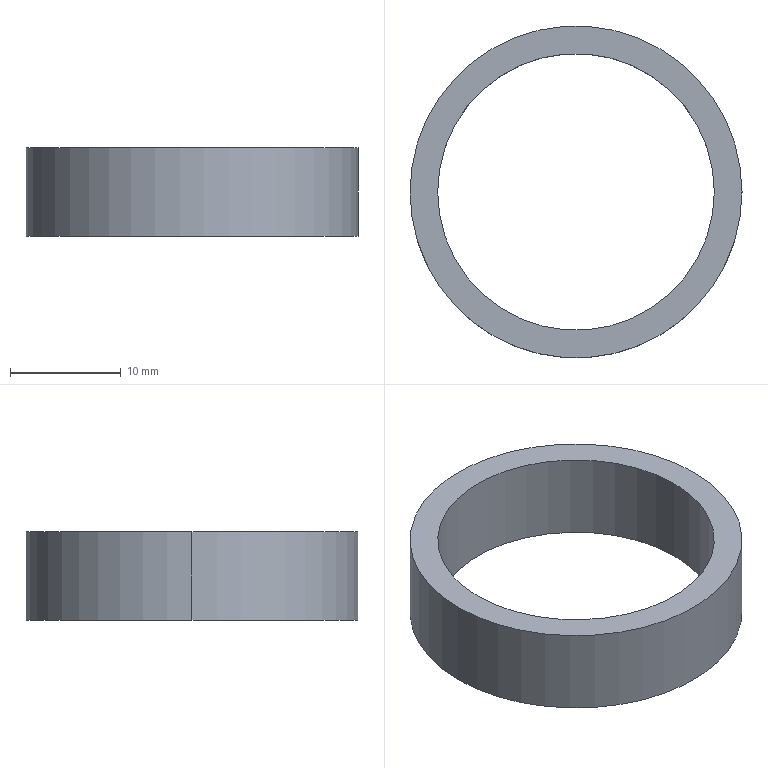Part | SolidWorks | features Extrusion 1 | 1 solid | 6 faces | box 30 x 30 x 8 mm | volume 1728 mm3 | cylinder 4 | plane 2 | commonest cylinder face diameters 25 x2 30 x2
STEP:
#1=CARTESIAN_POINT('',(-12.5,0.,8.));
#2=VERTEX_POINT('',#1);
#3=CARTESIAN_POINT('',(12.5,0.,8.));
#4=VERTEX_POINT('',#3);
#5=CARTESIAN_POINT('',(0.,0.,8.));
#6=DIRECTION('',(0.,0.,1.));
#7=DIRECTION('',(1.,0.,0.));
#8=AXIS2_PLACEMENT_3D('',#5,#6,#7);
#9=CIRCLE('',#8,12.5);
#10=EDGE_CURVE('',#2,#4,#9,.T.);
#11=ORIENTED_EDGE('',*,*,#10,.T.);
#12=CARTESIAN_POINT('',(12.5,0.,0.));
#13=VERTEX_POINT('',#12);
#14=CARTESIAN_POINT('',(12.5,0.,8.));
#15=DIRECTION('',(0.,0.,-1.));
#16=VECTOR('',#15,1000.);
#17=LINE('',#14,#16);
#18=EDGE_CURVE('',#4,#13,#17,.T.);
#19=ORIENTED_EDGE('',*,*,#18,.T.);
#20=CARTESIAN_POINT('',(-12.5,0.,0.));
#21=VERTEX_POINT('',#20);
#22=CARTESIAN_POINT('',(0.,0.,0.));
#23=DIRECTION('',(0.,0.,1.));
#24=DIRECTION('',(1.,0.,0.));
#25=AXIS2_PLACEMENT_3D('',#22,#23,#24);
#26=CIRCLE('',#25,12.5);
#27=EDGE_CURVE('',#21,#13,#26,.T.);
#28=ORIENTED_EDGE('',*,*,#27,.F.);
#29=CARTESIAN_POINT('',(-12.5,0.,8.));
#30=DIRECTION('',(0.,0.,-1.));
#31=VECTOR('',#30,1000.);
#32=LINE('',#29,#31);
#33=EDGE_CURVE('',#2,#21,#32,.T.);
#34=ORIENTED_EDGE('',*,*,#33,.F.);
#35=EDGE_LOOP('',(#11,#19,#28,#34));
#36=FACE_OUTER_BOUND('',#35,.T.);
#37=CARTESIAN_POINT('',(0.,0.,8.));
#38=DIRECTION('',(0.,0.,-1.));
#39=DIRECTION('',(-1.,0.,0.));
#40=AXIS2_PLACEMENT_3D('',#37,#38,#39);
#41=CYLINDRICAL_SURFACE('',#40,12.5);
#42=ADVANCED_FACE('',(#36),#41,.F.);
#43=CARTESIAN_POINT('',(15.,0.,8.));
#44=VERTEX_POINT('',#43);
#45=CARTESIAN_POINT('',(-15.,0.,8.));
#46=VERTEX_POINT('',#45);
#47=CARTESIAN_POINT('',(0.,0.,8.));
#48=DIRECTION('',(0.,0.,1.));
#49=DIRECTION('',(1.,0.,0.));
#50=AXIS2_PLACEMENT_3D('',#47,#48,#49);
#51=CIRCLE('',#50,15.);
#52=EDGE_CURVE('',#44,#46,#51,.T.);
#53=ORIENTED_EDGE('',*,*,#52,.F.);
#54=CARTESIAN_POINT('',(15.,0.,0.));
#55=VERTEX_POINT('',#54);
#56=CARTESIAN_POINT('',(15.,0.,8.));
#57=DIRECTION('',(0.,0.,-1.));
#58=VECTOR('',#57,1000.);
#59=LINE('',#56,#58);
#60=EDGE_CURVE('',#44,#55,#59,.T.);
#61=ORIENTED_EDGE('',*,*,#60,.T.);
#62=CARTESIAN_POINT('',(-15.,0.,0.));
#63=VERTEX_POINT('',#62);
#64=CARTESIAN_POINT('',(0.,0.,0.));
#65=DIRECTION('',(0.,0.,1.));
#66=DIRECTION('',(1.,0.,0.));
#67=AXIS2_PLACEMENT_3D('',#64,#65,#66);
#68=CIRCLE('',#67,15.);
#69=EDGE_CURVE('',#55,#63,#68,.T.);
#70=ORIENTED_EDGE('',*,*,#69,.T.);
#71=CARTESIAN_POINT('',(-15.,0.,8.));
#72=DIRECTION('',(0.,0.,-1.));
#73=VECTOR('',#72,1000.);
#74=LINE('',#71,#73);
#75=EDGE_CURVE('',#46,#63,#74,.T.);
#76=ORIENTED_EDGE('',*,*,#75,.F.);
#77=EDGE_LOOP('',(#53,#61,#70,#76));
#78=FACE_OUTER_BOUND('',#77,.T.);
#79=CARTESIAN_POINT('',(0.,0.,8.));
#80=DIRECTION('',(0.,0.,-1.));
#81=DIRECTION('',(-1.,0.,0.));
#82=AXIS2_PLACEMENT_3D('',#79,#80,#81);
#83=CYLINDRICAL_SURFACE('',#82,15.);
#84=ADVANCED_FACE('',(#78),#83,.T.);
#85=CARTESIAN_POINT('',(0.,0.,8.));
#86=DIRECTION('',(0.,0.,1.));
#87=DIRECTION('',(1.,0.,0.));
#88=AXIS2_PLACEMENT_3D('',#85,#86,#87);
#89=CIRCLE('',#88,15.);
#90=EDGE_CURVE('',#46,#44,#89,.T.);
#91=ORIENTED_EDGE('',*,*,#90,.T.);
#92=ORIENTED_EDGE('',*,*,#52,.T.);
#93=EDGE_LOOP('',(#91,#92));
#94=FACE_OUTER_BOUND('',#93,.T.);
#95=ORIENTED_EDGE('',*,*,#10,.F.);
#96=CARTESIAN_POINT('',(0.,0.,8.));
#97=DIRECTION('',(0.,0.,1.));
#98=DIRECTION('',(1.,0.,0.));
#99=AXIS2_PLACEMENT_3D('',#96,#97,#98);
#100=CIRCLE('',#99,12.5);
#101=EDGE_CURVE('',#4,#2,#100,.T.);
#102=ORIENTED_EDGE('',*,*,#101,.F.);
#103=EDGE_LOOP('',(#95,#102));
#104=FACE_BOUND('',#103,.T.);
#105=CARTESIAN_POINT('',(0.,0.,8.));
#106=DIRECTION('',(0.,0.,1.));
#107=DIRECTION('',(1.,0.,0.));
#108=AXIS2_PLACEMENT_3D('',#105,#106,#107);
#109=PLANE('',#108);
#110=ADVANCED_FACE('',(#94,#104),#109,.T.);
#111=CARTESIAN_POINT('',(0.,0.,0.));
#112=DIRECTION('',(0.,0.,1.));
#113=DIRECTION('',(1.,0.,0.));
#114=AXIS2_PLACEMENT_3D('',#111,#112,#113);
#115=CIRCLE('',#114,15.);
#116=EDGE_CURVE('',#63,#55,#115,.T.);
#117=ORIENTED_EDGE('',*,*,#116,.F.);
#118=ORIENTED_EDGE('',*,*,#69,.F.);
#119=EDGE_LOOP('',(#117,#118));
#120=FACE_OUTER_BOUND('',#119,.T.);
#121=ORIENTED_EDGE('',*,*,#27,.T.);
#122=CARTESIAN_POINT('',(0.,0.,0.));
#123=DIRECTION('',(0.,0.,1.));
#124=DIRECTION('',(1.,0.,0.));
#125=AXIS2_PLACEMENT_3D('',#122,#123,#124);
#126=CIRCLE('',#125,12.5);
#127=EDGE_CURVE('',#13,#21,#126,.T.);
#128=ORIENTED_EDGE('',*,*,#127,.T.);
#129=EDGE_LOOP('',(#121,#128));
#130=FACE_BOUND('',#129,.T.);
#131=CARTESIAN_POINT('',(0.,0.,0.));
#132=DIRECTION('',(0.,0.,1.));
#133=DIRECTION('',(1.,0.,0.));
#134=AXIS2_PLACEMENT_3D('',#131,#132,#133);
#135=PLANE('',#134);
#136=ADVANCED_FACE('',(#120,#130),#135,.F.);
#137=ORIENTED_EDGE('',*,*,#60,.F.);
#138=ORIENTED_EDGE('',*,*,#90,.F.);
#139=ORIENTED_EDGE('',*,*,#75,.T.);
#140=ORIENTED_EDGE('',*,*,#116,.T.);
#141=EDGE_LOOP('',(#137,#138,#139,#140));
#142=FACE_OUTER_BOUND('',#141,.T.);
#143=CARTESIAN_POINT('',(0.,0.,8.));
#144=DIRECTION('',(0.,0.,-1.));
#145=DIRECTION('',(-1.,0.,0.));
#146=AXIS2_PLACEMENT_3D('',#143,#144,#145);
#147=CYLINDRICAL_SURFACE('',#146,15.);
#148=ADVANCED_FACE('',(#142),#147,.T.);
#149=ORIENTED_EDGE('',*,*,#18,.F.);
#150=ORIENTED_EDGE('',*,*,#101,.T.);
#151=ORIENTED_EDGE('',*,*,#33,.T.);
#152=ORIENTED_EDGE('',*,*,#127,.F.);
#153=EDGE_LOOP('',(#149,#150,#151,#152));
#154=FACE_OUTER_BOUND('',#153,.T.);
#155=CARTESIAN_POINT('',(0.,0.,8.));
#156=DIRECTION('',(0.,0.,-1.));
#157=DIRECTION('',(-1.,0.,0.));
#158=AXIS2_PLACEMENT_3D('',#155,#156,#157);
#159=CYLINDRICAL_SURFACE('',#158,12.5);
#160=ADVANCED_FACE('',(#154),#159,.F.);
#161=CLOSED_SHELL('',(#42,#84,#110,#136,#148,#160));
#162=MANIFOLD_SOLID_BREP('',#161);
#163=CARTESIAN_POINT('',(0.,0.,0.));
#164=DIRECTION('',(0.,0.,1.));
#165=DIRECTION('',(1.,0.,0.));
#166=AXIS2_PLACEMENT_3D('',#163,#164,#165);
#167=(LENGTH_UNIT()NAMED_UNIT(*)SI_UNIT(.MILLI.,.METRE.));
#168=UNCERTAINTY_MEASURE_WITH_UNIT(LENGTH_MEASURE(0.00001),#167,'','');
#169=(NAMED_UNIT(*)PLANE_ANGLE_UNIT()SI_UNIT($,.RADIAN.));
#170=(NAMED_UNIT(*)SI_UNIT($,.STERADIAN.)SOLID_ANGLE_UNIT());
#171=(GEOMETRIC_REPRESENTATION_CONTEXT(3)GLOBAL_UNCERTAINTY_ASSIGNED_CONTEXT((#168))GLOBAL_UNIT_ASSIGNED_CONTEXT((#167,#169,#170))REPRESENTATION_CONTEXT('',''));
#172=ADVANCED_BREP_SHAPE_REPRESENTATION('',(#162,#166),#171);